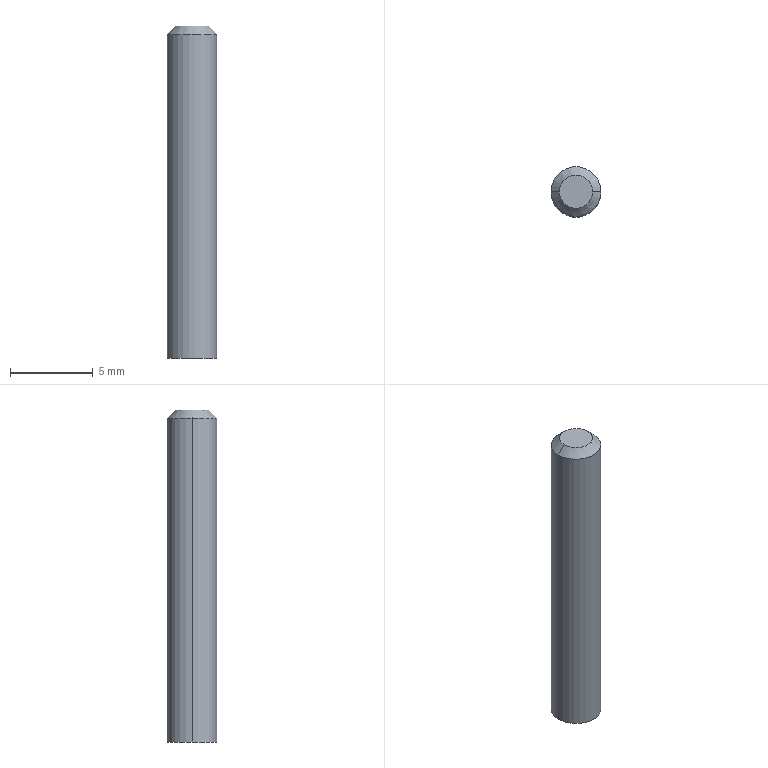Part | SolidWorks | features BaseBody 1 | 1 solid | 6 faces | box 3 x 3 x 20 mm | volume 140.324 mm3 | cylinder 2 | cone 2 | plane 2 | commonest cylinder face diameters 3 x2
STEP:
#1=CARTESIAN_POINT('',(12.189,6.319,0.));
#2=VERTEX_POINT('',#1);
#3=CARTESIAN_POINT('',(9.189,6.319,0.));
#4=VERTEX_POINT('',#3);
#5=CARTESIAN_POINT('',(10.689,6.319,0.));
#6=DIRECTION('',(0.,0.,1.));
#7=DIRECTION('',(1.,0.,0.));
#8=AXIS2_PLACEMENT_3D('',#5,#6,#7);
#9=CIRCLE('',#8,1.5);
#10=EDGE_CURVE('',#2,#4,#9,.T.);
#11=ORIENTED_EDGE('',*,*,#10,.T.);
#12=CARTESIAN_POINT('',(9.189,6.319,19.5));
#13=VERTEX_POINT('',#12);
#14=CARTESIAN_POINT('',(9.189,6.319,0.));
#15=DIRECTION('',(0.,0.,1.));
#16=VECTOR('',#15,1000.);
#17=LINE('',#14,#16);
#18=EDGE_CURVE('',#4,#13,#17,.T.);
#19=ORIENTED_EDGE('',*,*,#18,.T.);
#20=CARTESIAN_POINT('',(12.189,6.319,19.5));
#21=VERTEX_POINT('',#20);
#22=CARTESIAN_POINT('',(10.689,6.319,19.5));
#23=DIRECTION('',(0.,0.,-1.));
#24=DIRECTION('',(1.,0.,0.));
#25=AXIS2_PLACEMENT_3D('',#22,#23,#24);
#26=CIRCLE('',#25,1.5);
#27=EDGE_CURVE('',#13,#21,#26,.T.);
#28=ORIENTED_EDGE('',*,*,#27,.T.);
#29=CARTESIAN_POINT('',(12.189,6.319,0.));
#30=DIRECTION('',(0.,0.,1.));
#31=VECTOR('',#30,1000.);
#32=LINE('',#29,#31);
#33=EDGE_CURVE('',#2,#21,#32,.T.);
#34=ORIENTED_EDGE('',*,*,#33,.F.);
#35=EDGE_LOOP('',(#11,#19,#28,#34));
#36=FACE_OUTER_BOUND('',#35,.T.);
#37=CARTESIAN_POINT('',(10.689,6.319,0.));
#38=DIRECTION('',(0.,0.,1.));
#39=DIRECTION('',(1.,0.,0.));
#40=AXIS2_PLACEMENT_3D('',#37,#38,#39);
#41=CYLINDRICAL_SURFACE('',#40,1.5);
#42=ADVANCED_FACE('',(#36),#41,.T.);
#43=CARTESIAN_POINT('',(9.689,6.319,20.));
#44=VERTEX_POINT('',#43);
#45=CARTESIAN_POINT('',(11.689,6.319,20.));
#46=VERTEX_POINT('',#45);
#47=CARTESIAN_POINT('',(10.689,6.319,20.));
#48=DIRECTION('',(0.,0.,-1.));
#49=DIRECTION('',(-1.,0.,0.));
#50=AXIS2_PLACEMENT_3D('',#47,#48,#49);
#51=CIRCLE('',#50,1.);
#52=EDGE_CURVE('',#44,#46,#51,.T.);
#53=ORIENTED_EDGE('',*,*,#52,.T.);
#54=CARTESIAN_POINT('',(12.189,6.319,19.5));
#55=DIRECTION('',(0.7071,0.,-0.7071));
#56=VECTOR('',#55,1000.);
#57=LINE('',#54,#56);
#58=EDGE_CURVE('',#46,#21,#57,.T.);
#59=ORIENTED_EDGE('',*,*,#58,.T.);
#60=ORIENTED_EDGE('',*,*,#27,.F.);
#61=CARTESIAN_POINT('',(9.189,6.319,19.5));
#62=DIRECTION('',(-0.7071,0.,-0.7071));
#63=VECTOR('',#62,1000.);
#64=LINE('',#61,#63);
#65=EDGE_CURVE('',#44,#13,#64,.T.);
#66=ORIENTED_EDGE('',*,*,#65,.F.);
#67=EDGE_LOOP('',(#53,#59,#60,#66));
#68=FACE_OUTER_BOUND('',#67,.T.);
#69=CARTESIAN_POINT('',(10.689,6.319,19.5));
#70=DIRECTION('',(0.,0.,-1.));
#71=DIRECTION('',(-1.,0.,0.));
#72=AXIS2_PLACEMENT_3D('',#69,#70,#71);
#73=CONICAL_SURFACE('',#72,1.5,0.7854);
#74=ADVANCED_FACE('',(#68),#73,.T.);
#75=ORIENTED_EDGE('',*,*,#18,.F.);
#76=CARTESIAN_POINT('',(10.689,6.319,0.));
#77=DIRECTION('',(0.,0.,1.));
#78=DIRECTION('',(1.,0.,0.));
#79=AXIS2_PLACEMENT_3D('',#76,#77,#78);
#80=CIRCLE('',#79,1.5);
#81=EDGE_CURVE('',#4,#2,#80,.T.);
#82=ORIENTED_EDGE('',*,*,#81,.T.);
#83=ORIENTED_EDGE('',*,*,#33,.T.);
#84=CARTESIAN_POINT('',(10.689,6.319,19.5));
#85=DIRECTION('',(0.,0.,-1.));
#86=DIRECTION('',(1.,0.,0.));
#87=AXIS2_PLACEMENT_3D('',#84,#85,#86);
#88=CIRCLE('',#87,1.5);
#89=EDGE_CURVE('',#21,#13,#88,.T.);
#90=ORIENTED_EDGE('',*,*,#89,.T.);
#91=EDGE_LOOP('',(#75,#82,#83,#90));
#92=FACE_OUTER_BOUND('',#91,.T.);
#93=CARTESIAN_POINT('',(10.689,6.319,0.));
#94=DIRECTION('',(0.,0.,1.));
#95=DIRECTION('',(1.,0.,0.));
#96=AXIS2_PLACEMENT_3D('',#93,#94,#95);
#97=CYLINDRICAL_SURFACE('',#96,1.5);
#98=ADVANCED_FACE('',(#92),#97,.T.);
#99=ORIENTED_EDGE('',*,*,#58,.F.);
#100=CARTESIAN_POINT('',(10.689,6.319,20.));
#101=DIRECTION('',(0.,0.,-1.));
#102=DIRECTION('',(-1.,0.,0.));
#103=AXIS2_PLACEMENT_3D('',#100,#101,#102);
#104=CIRCLE('',#103,1.);
#105=EDGE_CURVE('',#46,#44,#104,.T.);
#106=ORIENTED_EDGE('',*,*,#105,.T.);
#107=ORIENTED_EDGE('',*,*,#65,.T.);
#108=ORIENTED_EDGE('',*,*,#89,.F.);
#109=EDGE_LOOP('',(#99,#106,#107,#108));
#110=FACE_OUTER_BOUND('',#109,.T.);
#111=CARTESIAN_POINT('',(10.689,6.319,19.5));
#112=DIRECTION('',(0.,0.,-1.));
#113=DIRECTION('',(-1.,0.,0.));
#114=AXIS2_PLACEMENT_3D('',#111,#112,#113);
#115=CONICAL_SURFACE('',#114,1.5,0.7854);
#116=ADVANCED_FACE('',(#110),#115,.T.);
#117=ORIENTED_EDGE('',*,*,#10,.F.);
#118=ORIENTED_EDGE('',*,*,#81,.F.);
#119=EDGE_LOOP('',(#117,#118));
#120=FACE_OUTER_BOUND('',#119,.T.);
#121=CARTESIAN_POINT('',(10.689,6.319,0.));
#122=DIRECTION('',(0.,0.,-1.));
#123=DIRECTION('',(-1.,0.,0.));
#124=AXIS2_PLACEMENT_3D('',#121,#122,#123);
#125=PLANE('',#124);
#126=ADVANCED_FACE('',(#120),#125,.T.);
#127=ORIENTED_EDGE('',*,*,#52,.F.);
#128=ORIENTED_EDGE('',*,*,#105,.F.);
#129=EDGE_LOOP('',(#127,#128));
#130=FACE_OUTER_BOUND('',#129,.T.);
#131=CARTESIAN_POINT('',(10.689,6.319,20.));
#132=DIRECTION('',(0.,0.,-1.));
#133=DIRECTION('',(-1.,0.,0.));
#134=AXIS2_PLACEMENT_3D('',#131,#132,#133);
#135=PLANE('',#134);
#136=ADVANCED_FACE('',(#130),#135,.F.);
#137=CLOSED_SHELL('',(#42,#74,#98,#116,#126,#136));
#138=MANIFOLD_SOLID_BREP('',#137);
#139=CARTESIAN_POINT('',(0.,0.,0.));
#140=DIRECTION('',(0.,0.,1.));
#141=DIRECTION('',(1.,0.,0.));
#142=AXIS2_PLACEMENT_3D('',#139,#140,#141);
#143=(LENGTH_UNIT()NAMED_UNIT(*)SI_UNIT(.MILLI.,.METRE.));
#144=UNCERTAINTY_MEASURE_WITH_UNIT(LENGTH_MEASURE(0.00001),#143,'','');
#145=(NAMED_UNIT(*)PLANE_ANGLE_UNIT()SI_UNIT($,.RADIAN.));
#146=(NAMED_UNIT(*)SI_UNIT($,.STERADIAN.)SOLID_ANGLE_UNIT());
#147=(GEOMETRIC_REPRESENTATION_CONTEXT(3)GLOBAL_UNCERTAINTY_ASSIGNED_CONTEXT((#144))GLOBAL_UNIT_ASSIGNED_CONTEXT((#143,#145,#146))REPRESENTATION_CONTEXT('',''));
#148=ADVANCED_BREP_SHAPE_REPRESENTATION('',(#138,#142),#147);